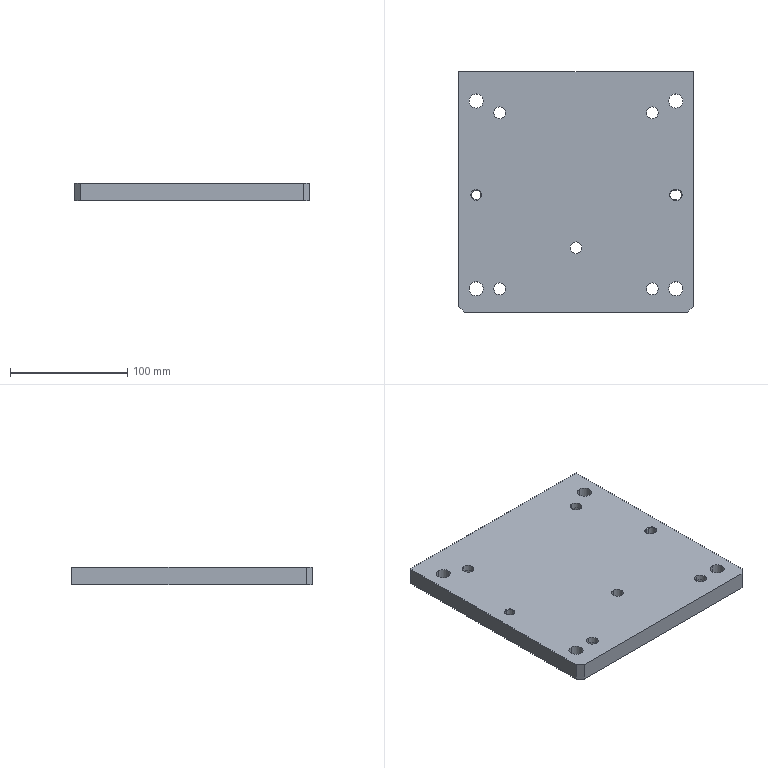Part | STEP file | J453-EBZ05-01-04-Part-1 | 1 solid | 88 faces | box 200 x 205 x 15 mm | volume 591806 mm3 | cylinder 46 | plane 22 | cone 20 | commonest cylinder face diameters 8 x12 10 x10 12 x8 16 x8 6.9 x4 7.5 x4